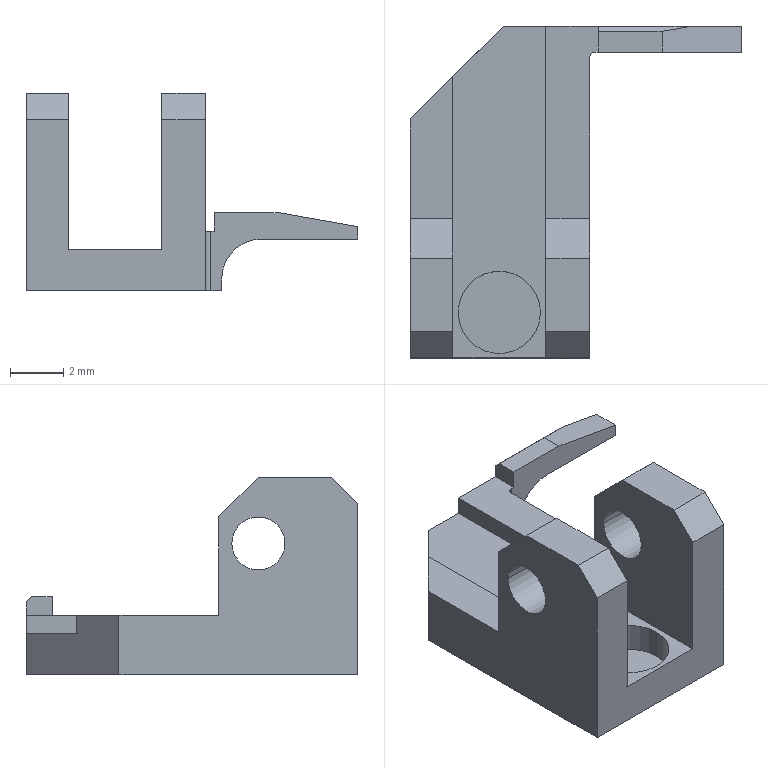Part | NX | 1 solid | 36 faces | box 12.481 x 12.5 x 7.45 mm | volume 217.887 mm3 | plane 28 | cylinder 8 | commonest cylinder face diameters 2 x4 3.1 x2 0.4 x1 3 x1
STEP:
#1=CARTESIAN_POINT('',(-42.479,-42.729,-0.8259));
#2=VERTEX_POINT('',#1);
#3=CARTESIAN_POINT('',(-42.479,-43.716,-0.8259));
#4=VERTEX_POINT('',#3);
#5=CARTESIAN_POINT('',(-42.479,-43.322,-0.8259));
#6=DIRECTION('',(0.,-1.,0.));
#7=VECTOR('',#6,1000.);
#8=LINE('',#5,#7);
#9=EDGE_CURVE('',#2,#4,#8,.T.);
#10=ORIENTED_EDGE('',*,*,#9,.T.);
#11=CARTESIAN_POINT('',(-42.479,-43.716,-1.297));
#12=VERTEX_POINT('',#11);
#13=CARTESIAN_POINT('',(-42.479,-43.716,-2.097));
#14=DIRECTION('',(0.,0.,1.));
#15=VECTOR('',#14,1000.);
#16=LINE('',#13,#15);
#17=EDGE_CURVE('',#12,#4,#16,.T.);
#18=ORIENTED_EDGE('',*,*,#17,.F.);
#19=CARTESIAN_POINT('',(-42.479,-42.729,-1.297));
#20=VERTEX_POINT('',#19);
#21=CARTESIAN_POINT('',(-42.479,-42.161,-1.297));
#22=DIRECTION('',(0.,1.,0.));
#23=VECTOR('',#22,1000.);
#24=LINE('',#21,#23);
#25=EDGE_CURVE('',#12,#20,#24,.T.);
#26=ORIENTED_EDGE('',*,*,#25,.T.);
#27=CARTESIAN_POINT('',(-42.479,-42.729,-2.097));
#28=DIRECTION('',(0.,0.,-1.));
#29=VECTOR('',#28,1000.);
#30=LINE('',#27,#29);
#31=EDGE_CURVE('',#2,#20,#30,.T.);
#32=ORIENTED_EDGE('',*,*,#31,.F.);
#33=EDGE_LOOP('',(#10,#18,#26,#32));
#34=FACE_BOUND('',#33,.T.);
#35=CARTESIAN_POINT('',(-42.479,-43.677,-2.097));
#36=DIRECTION('',(1.,0.,0.));
#37=DIRECTION('',(0.,0.,1.));
#38=AXIS2_PLACEMENT_3D('',#35,#36,#37);
#39=PLANE('',#38);
#40=ADVANCED_FACE('',(#34),#39,.T.);
#41=CARTESIAN_POINT('',(-47.879,-43.716,-0.9969));
#42=VERTEX_POINT('',#41);
#43=CARTESIAN_POINT('',(-47.879,-43.716,-0.2969));
#44=VERTEX_POINT('',#43);
#45=CARTESIAN_POINT('',(-47.879,-43.716,-2.097));
#46=DIRECTION('',(0.,0.,1.));
#47=VECTOR('',#46,1000.);
#48=LINE('',#45,#47);
#49=EDGE_CURVE('',#42,#44,#48,.T.);
#50=ORIENTED_EDGE('',*,*,#49,.T.);
#51=CARTESIAN_POINT('',(-47.879,-42.929,-0.2969));
#52=VERTEX_POINT('',#51);
#53=CARTESIAN_POINT('',(-47.879,-42.161,-0.2969));
#54=DIRECTION('',(0.,-1.,0.));
#55=VECTOR('',#54,1000.);
#56=LINE('',#53,#55);
#57=EDGE_CURVE('',#52,#44,#56,.T.);
#58=ORIENTED_EDGE('',*,*,#57,.F.);
#59=CARTESIAN_POINT('',(-47.879,-42.729,-0.4969));
#60=VERTEX_POINT('',#59);
#61=CARTESIAN_POINT('',(-47.879,-42.161,-1.065));
#62=DIRECTION('',(0.,0.7071,-0.7071));
#63=VECTOR('',#62,1000.);
#64=LINE('',#61,#63);
#65=EDGE_CURVE('',#52,#60,#64,.T.);
#66=ORIENTED_EDGE('',*,*,#65,.T.);
#67=CARTESIAN_POINT('',(-47.879,-42.729,-0.9969));
#68=VERTEX_POINT('',#67);
#69=CARTESIAN_POINT('',(-47.879,-42.729,-2.097));
#70=DIRECTION('',(0.,0.,-1.));
#71=VECTOR('',#70,1000.);
#72=LINE('',#69,#71);
#73=EDGE_CURVE('',#60,#68,#72,.T.);
#74=ORIENTED_EDGE('',*,*,#73,.T.);
#75=CARTESIAN_POINT('',(-47.879,-42.161,-0.9969));
#76=DIRECTION('',(0.,-1.,0.));
#77=VECTOR('',#76,1000.);
#78=LINE('',#75,#77);
#79=EDGE_CURVE('',#68,#42,#78,.T.);
#80=ORIENTED_EDGE('',*,*,#79,.T.);
#81=EDGE_LOOP('',(#50,#58,#66,#74,#80));
#82=FACE_BOUND('',#81,.T.);
#83=CARTESIAN_POINT('',(-47.879,-42.677,-2.097));
#84=DIRECTION('',(-1.,0.,0.));
#85=DIRECTION('',(0.,1.,0.));
#86=AXIS2_PLACEMENT_3D('',#83,#84,#85);
#87=PLANE('',#86);
#88=ADVANCED_FACE('',(#82),#87,.T.);
#89=CARTESIAN_POINT('',(-53.36,-55.229,-1.697));
#90=VERTEX_POINT('',#89);
#91=CARTESIAN_POINT('',(-53.36,-55.229,3.203));
#92=VERTEX_POINT('',#91);
#93=CARTESIAN_POINT('',(-53.36,-55.229,-2.097));
#94=DIRECTION('',(0.,0.,1.));
#95=VECTOR('',#94,1000.);
#96=LINE('',#93,#95);
#97=EDGE_CURVE('',#90,#92,#96,.T.);
#98=ORIENTED_EDGE('',*,*,#97,.F.);
#99=CARTESIAN_POINT('',(-53.36,-44.629,-1.697));
#100=VERTEX_POINT('',#99);
#101=CARTESIAN_POINT('',(-53.36,-42.161,-1.697));
#102=DIRECTION('',(0.,-1.,0.));
#103=VECTOR('',#102,1000.);
#104=LINE('',#101,#103);
#105=EDGE_CURVE('',#100,#90,#104,.T.);
#106=ORIENTED_EDGE('',*,*,#105,.F.);
#107=CARTESIAN_POINT('',(-53.36,-44.629,-0.9969));
#108=VERTEX_POINT('',#107);
#109=CARTESIAN_POINT('',(-53.36,-44.629,-2.097));
#110=DIRECTION('',(0.,0.,-1.));
#111=VECTOR('',#110,1000.);
#112=LINE('',#109,#111);
#113=EDGE_CURVE('',#108,#100,#112,.T.);
#114=ORIENTED_EDGE('',*,*,#113,.F.);
#115=CARTESIAN_POINT('',(-53.36,-49.979,-0.9969));
#116=VERTEX_POINT('',#115);
#117=CARTESIAN_POINT('',(-53.36,-42.161,-0.9969));
#118=DIRECTION('',(0.,-1.,0.));
#119=VECTOR('',#118,1000.);
#120=LINE('',#117,#119);
#121=EDGE_CURVE('',#108,#116,#120,.T.);
#122=ORIENTED_EDGE('',*,*,#121,.T.);
#123=CARTESIAN_POINT('',(-53.36,-49.979,2.703));
#124=VERTEX_POINT('',#123);
#125=CARTESIAN_POINT('',(-53.36,-49.979,-2.097));
#126=DIRECTION('',(0.,0.,-1.));
#127=VECTOR('',#126,1000.);
#128=LINE('',#125,#127);
#129=EDGE_CURVE('',#124,#116,#128,.T.);
#130=ORIENTED_EDGE('',*,*,#129,.F.);
#131=CARTESIAN_POINT('',(-53.36,-51.479,4.203));
#132=VERTEX_POINT('',#131);
#133=CARTESIAN_POINT('',(-53.36,-45.179,-2.097));
#134=DIRECTION('',(0.,-0.7071,0.7071));
#135=VECTOR('',#134,1000.);
#136=LINE('',#133,#135);
#137=EDGE_CURVE('',#124,#132,#136,.T.);
#138=ORIENTED_EDGE('',*,*,#137,.T.);
#139=CARTESIAN_POINT('',(-53.36,-54.229,4.203));
#140=VERTEX_POINT('',#139);
#141=CARTESIAN_POINT('',(-53.36,-42.161,4.203));
#142=DIRECTION('',(0.,1.,0.));
#143=VECTOR('',#142,1000.);
#144=LINE('',#141,#143);
#145=EDGE_CURVE('',#140,#132,#144,.T.);
#146=ORIENTED_EDGE('',*,*,#145,.F.);
#147=CARTESIAN_POINT('',(-53.36,-60.529,-2.097));
#148=DIRECTION('',(0.,-0.7071,-0.7071));
#149=VECTOR('',#148,1000.);
#150=LINE('',#147,#149);
#151=EDGE_CURVE('',#140,#92,#150,.T.);
#152=ORIENTED_EDGE('',*,*,#151,.T.);
#153=EDGE_LOOP('',(#98,#106,#114,#122,#130,#138,#146,#152));
#154=FACE_BOUND('',#153,.T.);
#155=CARTESIAN_POINT('',(-53.36,-52.479,1.703));
#156=VERTEX_POINT('',#155);
#157=CARTESIAN_POINT('',(-53.36,-50.479,1.703));
#158=VERTEX_POINT('',#157);
#159=CARTESIAN_POINT('',(-53.36,-51.479,1.703));
#160=DIRECTION('',(-1.,0.,0.));
#161=DIRECTION('',(0.,-1.,0.));
#162=AXIS2_PLACEMENT_3D('',#159,#160,#161);
#163=CIRCLE('',#162,1.);
#164=EDGE_CURVE('',#156,#158,#163,.T.);
#165=ORIENTED_EDGE('',*,*,#164,.T.);
#166=CARTESIAN_POINT('',(-53.36,-51.479,1.703));
#167=DIRECTION('',(-1.,0.,0.));
#168=DIRECTION('',(0.,-1.,0.));
#169=AXIS2_PLACEMENT_3D('',#166,#167,#168);
#170=CIRCLE('',#169,1.);
#171=EDGE_CURVE('',#158,#156,#170,.T.);
#172=ORIENTED_EDGE('',*,*,#171,.T.);
#173=EDGE_LOOP('',(#165,#172));
#174=FACE_BOUND('',#173,.T.);
#175=CARTESIAN_POINT('',(-53.36,-41.455,-0.9969));
#176=DIRECTION('',(-1.,0.,0.));
#177=DIRECTION('',(0.,0.,1.));
#178=AXIS2_PLACEMENT_3D('',#175,#176,#177);
#179=PLANE('',#178);
#180=ADVANCED_FACE('',(#154,#174),#179,.F.);
#181=ORIENTED_EDGE('',*,*,#31,.T.);
#182=CARTESIAN_POINT('',(-46.102,-42.729,-1.297));
#183=VERTEX_POINT('',#182);
#184=CARTESIAN_POINT('',(-49.458,-42.729,-1.297));
#185=DIRECTION('',(-1.,0.,0.));
#186=VECTOR('',#185,1000.);
#187=LINE('',#184,#186);
#188=EDGE_CURVE('',#20,#183,#187,.T.);
#189=ORIENTED_EDGE('',*,*,#188,.T.);
#190=CARTESIAN_POINT('',(-47.602,-42.729,-2.797));
#191=VERTEX_POINT('',#190);
#192=CARTESIAN_POINT('',(-46.102,-42.729,-2.797));
#193=DIRECTION('',(0.,1.,0.));
#194=DIRECTION('',(0.,0.,-1.));
#195=AXIS2_PLACEMENT_3D('',#192,#193,#194);
#196=CIRCLE('',#195,1.5);
#197=EDGE_CURVE('',#191,#183,#196,.T.);
#198=ORIENTED_EDGE('',*,*,#197,.F.);
#199=CARTESIAN_POINT('',(-47.602,-42.729,-3.247));
#200=VERTEX_POINT('',#199);
#201=CARTESIAN_POINT('',(-47.602,-42.729,-2.097));
#202=DIRECTION('',(0.,0.,1.));
#203=VECTOR('',#202,1000.);
#204=LINE('',#201,#203);
#205=EDGE_CURVE('',#200,#191,#204,.T.);
#206=ORIENTED_EDGE('',*,*,#205,.F.);
#207=CARTESIAN_POINT('',(-51.46,-42.729,-3.247));
#208=VERTEX_POINT('',#207);
#209=CARTESIAN_POINT('',(-49.458,-42.729,-3.247));
#210=DIRECTION('',(-1.,0.,0.));
#211=VECTOR('',#210,1000.);
#212=LINE('',#209,#211);
#213=EDGE_CURVE('',#200,#208,#212,.T.);
#214=ORIENTED_EDGE('',*,*,#213,.T.);
#215=CARTESIAN_POINT('',(-51.46,-42.729,-1.697));
#216=VERTEX_POINT('',#215);
#217=CARTESIAN_POINT('',(-51.46,-42.729,-2.097));
#218=DIRECTION('',(0.,0.,1.));
#219=VECTOR('',#218,1000.);
#220=LINE('',#217,#219);
#221=EDGE_CURVE('',#208,#216,#220,.T.);
#222=ORIENTED_EDGE('',*,*,#221,.T.);
#223=CARTESIAN_POINT('',(-49.86,-42.729,-1.697));
#224=VERTEX_POINT('',#223);
#225=CARTESIAN_POINT('',(-49.458,-42.729,-1.697));
#226=DIRECTION('',(-1.,0.,0.));
#227=VECTOR('',#226,1000.);
#228=LINE('',#225,#227);
#229=EDGE_CURVE('',#224,#216,#228,.T.);
#230=ORIENTED_EDGE('',*,*,#229,.F.);
#231=CARTESIAN_POINT('',(-49.86,-42.729,-0.9969));
#232=VERTEX_POINT('',#231);
#233=CARTESIAN_POINT('',(-49.86,-42.729,-2.097));
#234=DIRECTION('',(0.,0.,-1.));
#235=VECTOR('',#234,1000.);
#236=LINE('',#233,#235);
#237=EDGE_CURVE('',#232,#224,#236,.T.);
#238=ORIENTED_EDGE('',*,*,#237,.F.);
#239=CARTESIAN_POINT('',(-49.458,-42.729,-0.9969));
#240=DIRECTION('',(-1.,0.,0.));
#241=VECTOR('',#240,1000.);
#242=LINE('',#239,#241);
#243=EDGE_CURVE('',#68,#232,#242,.T.);
#244=ORIENTED_EDGE('',*,*,#243,.F.);
#245=ORIENTED_EDGE('',*,*,#73,.F.);
#246=CARTESIAN_POINT('',(-44.345,-42.729,-0.4969));
#247=VERTEX_POINT('',#246);
#248=CARTESIAN_POINT('',(-49.458,-42.729,-0.4969));
#249=DIRECTION('',(1.,0.,0.));
#250=VECTOR('',#249,1000.);
#251=LINE('',#248,#250);
#252=EDGE_CURVE('',#60,#247,#251,.T.);
#253=ORIENTED_EDGE('',*,*,#252,.T.);
#254=CARTESIAN_POINT('',(-49.458,-42.729,0.4047));
#255=DIRECTION('',(0.9848,0.,-0.1736));
#256=VECTOR('',#255,1000.);
#257=LINE('',#254,#256);
#258=EDGE_CURVE('',#247,#2,#257,.T.);
#259=ORIENTED_EDGE('',*,*,#258,.T.);
#260=EDGE_LOOP('',(#181,#189,#198,#206,#214,#222,#230,#238,#244,#245,#253,#259));
#261=FACE_BOUND('',#260,.T.);
#262=CARTESIAN_POINT('',(-40.479,-42.729,-2.097));
#263=DIRECTION('',(0.,1.,0.));
#264=DIRECTION('',(0.,0.,-1.));
#265=AXIS2_PLACEMENT_3D('',#262,#263,#264);
#266=PLANE('',#265);
#267=ADVANCED_FACE('',(#261),#266,.T.);
#268=CARTESIAN_POINT('',(-48.01,-43.716,-0.9969));
#269=VERTEX_POINT('',#268);
#270=CARTESIAN_POINT('',(-48.01,-43.716,-3.247));
#271=VERTEX_POINT('',#270);
#272=CARTESIAN_POINT('',(-48.01,-43.716,-2.097));
#273=DIRECTION('',(0.,0.,-1.));
#274=VECTOR('',#273,1000.);
#275=LINE('',#272,#274);
#276=EDGE_CURVE('',#269,#271,#275,.T.);
#277=ORIENTED_EDGE('',*,*,#276,.T.);
#278=CARTESIAN_POINT('',(-47.602,-43.716,-3.247));
#279=VERTEX_POINT('',#278);
#280=CARTESIAN_POINT('',(-49.458,-43.716,-3.247));
#281=DIRECTION('',(1.,0.,0.));
#282=VECTOR('',#281,1000.);
#283=LINE('',#280,#282);
#284=EDGE_CURVE('',#271,#279,#283,.T.);
#285=ORIENTED_EDGE('',*,*,#284,.T.);
#286=CARTESIAN_POINT('',(-47.602,-43.716,-2.797));
#287=VERTEX_POINT('',#286);
#288=CARTESIAN_POINT('',(-47.602,-43.716,-2.097));
#289=DIRECTION('',(0.,0.,-1.));
#290=VECTOR('',#289,1000.);
#291=LINE('',#288,#290);
#292=EDGE_CURVE('',#287,#279,#291,.T.);
#293=ORIENTED_EDGE('',*,*,#292,.F.);
#294=CARTESIAN_POINT('',(-46.102,-43.716,-1.297));
#295=VERTEX_POINT('',#294);
#296=CARTESIAN_POINT('',(-46.102,-43.716,-2.797));
#297=DIRECTION('',(0.,-1.,0.));
#298=DIRECTION('',(0.,0.,1.));
#299=AXIS2_PLACEMENT_3D('',#296,#297,#298);
#300=CIRCLE('',#299,1.5);
#301=EDGE_CURVE('',#295,#287,#300,.T.);
#302=ORIENTED_EDGE('',*,*,#301,.F.);
#303=CARTESIAN_POINT('',(-49.458,-43.716,-1.297));
#304=DIRECTION('',(1.,0.,0.));
#305=VECTOR('',#304,1000.);
#306=LINE('',#303,#305);
#307=EDGE_CURVE('',#295,#12,#306,.T.);
#308=ORIENTED_EDGE('',*,*,#307,.T.);
#309=ORIENTED_EDGE('',*,*,#17,.T.);
#310=CARTESIAN_POINT('',(-45.479,-43.716,-0.2969));
#311=VERTEX_POINT('',#310);
#312=CARTESIAN_POINT('',(-49.458,-43.716,0.4047));
#313=DIRECTION('',(-0.9848,0.,0.1736));
#314=VECTOR('',#313,1000.);
#315=LINE('',#312,#314);
#316=EDGE_CURVE('',#4,#311,#315,.T.);
#317=ORIENTED_EDGE('',*,*,#316,.T.);
#318=CARTESIAN_POINT('',(-49.458,-43.716,-0.2969));
#319=DIRECTION('',(-1.,0.,0.));
#320=VECTOR('',#319,1000.);
#321=LINE('',#318,#320);
#322=EDGE_CURVE('',#311,#44,#321,.T.);
#323=ORIENTED_EDGE('',*,*,#322,.T.);
#324=ORIENTED_EDGE('',*,*,#49,.F.);
#325=CARTESIAN_POINT('',(-49.458,-43.716,-0.9969));
#326=DIRECTION('',(1.,0.,0.));
#327=VECTOR('',#326,1000.);
#328=LINE('',#325,#327);
#329=EDGE_CURVE('',#269,#42,#328,.T.);
#330=ORIENTED_EDGE('',*,*,#329,.F.);
#331=EDGE_LOOP('',(#277,#285,#293,#302,#308,#309,#317,#323,#324,#330));
#332=FACE_BOUND('',#331,.T.);
#333=CARTESIAN_POINT('',(-49.857,-43.716,-2.975));
#334=DIRECTION('',(0.,-1.,0.));
#335=DIRECTION('',(-1.,0.,0.));
#336=AXIS2_PLACEMENT_3D('',#333,#334,#335);
#337=PLANE('',#336);
#338=ADVANCED_FACE('',(#332),#337,.T.);
#339=CARTESIAN_POINT('',(-48.21,-55.229,-3.247));
#340=VERTEX_POINT('',#339);
#341=CARTESIAN_POINT('',(-48.21,-55.229,3.203));
#342=VERTEX_POINT('',#341);
#343=CARTESIAN_POINT('',(-48.21,-55.229,-2.097));
#344=DIRECTION('',(0.,0.,1.));
#345=VECTOR('',#344,1000.);
#346=LINE('',#343,#345);
#347=EDGE_CURVE('',#340,#342,#346,.T.);
#348=ORIENTED_EDGE('',*,*,#347,.T.);
#349=CARTESIAN_POINT('',(-49.86,-55.229,3.203));
#350=VERTEX_POINT('',#349);
#351=CARTESIAN_POINT('',(-49.035,-55.229,3.203));
#352=DIRECTION('',(1.,0.,0.));
#353=VECTOR('',#352,1000.);
#354=LINE('',#351,#353);
#355=EDGE_CURVE('',#350,#342,#354,.T.);
#356=ORIENTED_EDGE('',*,*,#355,.F.);
#357=CARTESIAN_POINT('',(-49.86,-55.229,-1.697));
#358=VERTEX_POINT('',#357);
#359=CARTESIAN_POINT('',(-49.86,-55.229,-2.097));
#360=DIRECTION('',(0.,0.,-1.));
#361=VECTOR('',#360,1000.);
#362=LINE('',#359,#361);
#363=EDGE_CURVE('',#350,#358,#362,.T.);
#364=ORIENTED_EDGE('',*,*,#363,.T.);
#365=CARTESIAN_POINT('',(-49.458,-55.229,-1.697));
#366=DIRECTION('',(-1.,0.,0.));
#367=VECTOR('',#366,1000.);
#368=LINE('',#365,#367);
#369=EDGE_CURVE('',#358,#90,#368,.T.);
#370=ORIENTED_EDGE('',*,*,#369,.T.);
#371=ORIENTED_EDGE('',*,*,#97,.T.);
#372=CARTESIAN_POINT('',(-54.96,-55.229,3.203));
#373=VERTEX_POINT('',#372);
#374=CARTESIAN_POINT('',(-54.16,-55.229,3.203));
#375=DIRECTION('',(1.,0.,0.));
#376=VECTOR('',#375,1000.);
#377=LINE('',#374,#376);
#378=EDGE_CURVE('',#373,#92,#377,.T.);
#379=ORIENTED_EDGE('',*,*,#378,.F.);
#380=CARTESIAN_POINT('',(-54.96,-55.229,-3.247));
#381=VERTEX_POINT('',#380);
#382=CARTESIAN_POINT('',(-54.96,-55.229,-2.097));
#383=DIRECTION('',(0.,0.,1.));
#384=VECTOR('',#383,1000.);
#385=LINE('',#382,#384);
#386=EDGE_CURVE('',#381,#373,#385,.T.);
#387=ORIENTED_EDGE('',*,*,#386,.F.);
#388=CARTESIAN_POINT('',(-49.458,-55.229,-3.247));
#389=DIRECTION('',(-1.,0.,0.));
#390=VECTOR('',#389,1000.);
#391=LINE('',#388,#390);
#392=EDGE_CURVE('',#340,#381,#391,.T.);
#393=ORIENTED_EDGE('',*,*,#392,.F.);
#394=EDGE_LOOP('',(#348,#356,#364,#370,#371,#379,#387,#393));
#395=FACE_BOUND('',#394,.T.);
#396=CARTESIAN_POINT('',(-46.479,-55.229,-2.097));
#397=DIRECTION('',(0.,-1.,0.));
#398=DIRECTION('',(-1.,0.,0.));
#399=AXIS2_PLACEMENT_3D('',#396,#397,#398);
#400=PLANE('',#399);
#401=ADVANCED_FACE('',(#395),#400,.T.);
#402=CARTESIAN_POINT('',(-47.602,-45.216,-2.797));
#403=DIRECTION('',(0.,1.,0.));
#404=VECTOR('',#403,1000.);
#405=LINE('',#402,#404);
#406=EDGE_CURVE('',#287,#191,#405,.T.);
#407=ORIENTED_EDGE('',*,*,#406,.F.);
#408=ORIENTED_EDGE('',*,*,#292,.T.);
#409=CARTESIAN_POINT('',(-47.602,-42.161,-3.247));
#410=DIRECTION('',(0.,-1.,0.));
#411=VECTOR('',#410,1000.);
#412=LINE('',#409,#411);
#413=EDGE_CURVE('',#200,#279,#412,.T.);
#414=ORIENTED_EDGE('',*,*,#413,.F.);
#415=ORIENTED_EDGE('',*,*,#205,.T.);
#416=EDGE_LOOP('',(#407,#408,#414,#415));
#417=FACE_BOUND('',#416,.T.);
#418=CARTESIAN_POINT('',(-47.602,-42.161,-2.747));
#419=DIRECTION('',(-1.,0.,0.));
#420=DIRECTION('',(0.,0.,1.));
#421=AXIS2_PLACEMENT_3D('',#418,#419,#420);
#422=PLANE('',#421);
#423=ADVANCED_FACE('',(#417),#422,.F.);
#424=ORIENTED_EDGE('',*,*,#406,.T.);
#425=ORIENTED_EDGE('',*,*,#197,.T.);
#426=CARTESIAN_POINT('',(-46.102,-45.216,-1.297));
#427=DIRECTION('',(0.,1.,0.));
#428=VECTOR('',#427,1000.);
#429=LINE('',#426,#428);
#430=EDGE_CURVE('',#295,#183,#429,.T.);
#431=ORIENTED_EDGE('',*,*,#430,.F.);
#432=ORIENTED_EDGE('',*,*,#301,.T.);
#433=EDGE_LOOP('',(#424,#425,#431,#432));
#434=FACE_BOUND('',#433,.T.);
#435=CARTESIAN_POINT('',(-46.102,-45.216,-2.797));
#436=DIRECTION('',(0.,1.,0.));
#437=DIRECTION('',(1.,0.,0.));
#438=AXIS2_PLACEMENT_3D('',#435,#436,#437);
#439=CYLINDRICAL_SURFACE('',#438,1.5);
#440=ADVANCED_FACE('',(#434),#439,.F.);
#441=ORIENTED_EDGE('',*,*,#276,.F.);
#442=CARTESIAN_POINT('',(-48.21,-43.916,-0.9969));
#443=VERTEX_POINT('',#442);
#444=CARTESIAN_POINT('',(-48.01,-43.916,-0.9969));
#445=DIRECTION('',(0.,0.,-1.));
#446=DIRECTION('',(-1.,0.,0.));
#447=AXIS2_PLACEMENT_3D('',#444,#445,#446);
#448=CIRCLE('',#447,0.2);
#449=EDGE_CURVE('',#443,#269,#448,.T.);
#450=ORIENTED_EDGE('',*,*,#449,.F.);
#451=CARTESIAN_POINT('',(-48.21,-43.916,-3.247));
#452=VERTEX_POINT('',#451);
#453=CARTESIAN_POINT('',(-48.21,-43.916,-2.097));
#454=DIRECTION('',(0.,0.,-1.));
#455=VECTOR('',#454,1000.);
#456=LINE('',#453,#455);
#457=EDGE_CURVE('',#443,#452,#456,.T.);
#458=ORIENTED_EDGE('',*,*,#457,.T.);
#459=CARTESIAN_POINT('',(-48.01,-43.916,-3.247));
#460=DIRECTION('',(0.,0.,-1.));
#461=DIRECTION('',(-1.,0.,0.));
#462=AXIS2_PLACEMENT_3D('',#459,#460,#461);
#463=CIRCLE('',#462,0.2);
#464=EDGE_CURVE('',#452,#271,#463,.T.);
#465=ORIENTED_EDGE('',*,*,#464,.T.);
#466=EDGE_LOOP('',(#441,#450,#458,#465));
#467=FACE_BOUND('',#466,.T.);
#468=CARTESIAN_POINT('',(-48.01,-43.916,-2.097));
#469=DIRECTION('',(0.,0.,-1.));
#470=DIRECTION('',(-1.,0.,0.));
#471=AXIS2_PLACEMENT_3D('',#468,#469,#470);
#472=CYLINDRICAL_SURFACE('',#471,0.2);
#473=ADVANCED_FACE('',(#467),#472,.F.);
#474=ORIENTED_EDGE('',*,*,#164,.F.);
#475=CARTESIAN_POINT('',(-54.96,-52.479,1.703));
#476=VERTEX_POINT('',#475);
#477=CARTESIAN_POINT('',(-40.131,-52.479,1.703));
#478=DIRECTION('',(-1.,0.,0.));
#479=VECTOR('',#478,1000.);
#480=LINE('',#477,#479);
#481=EDGE_CURVE('',#476,#156,#480,.F.);
#482=ORIENTED_EDGE('',*,*,#481,.F.);
#483=CARTESIAN_POINT('',(-54.96,-50.479,1.703));
#484=VERTEX_POINT('',#483);
#485=CARTESIAN_POINT('',(-54.96,-51.479,1.703));
#486=DIRECTION('',(-1.,0.,0.));
#487=DIRECTION('',(0.,-1.,0.));
#488=AXIS2_PLACEMENT_3D('',#485,#486,#487);
#489=CIRCLE('',#488,1.);
#490=EDGE_CURVE('',#476,#484,#489,.T.);
#491=ORIENTED_EDGE('',*,*,#490,.T.);
#492=CARTESIAN_POINT('',(-40.131,-50.479,1.703));
#493=DIRECTION('',(-1.,0.,0.));
#494=VECTOR('',#493,1000.);
#495=LINE('',#492,#494);
#496=EDGE_CURVE('',#484,#158,#495,.F.);
#497=ORIENTED_EDGE('',*,*,#496,.T.);
#498=EDGE_LOOP('',(#474,#482,#491,#497));
#499=FACE_BOUND('',#498,.T.);
#500=CARTESIAN_POINT('',(-40.131,-51.479,1.703));
#501=DIRECTION('',(-1.,0.,0.));
#502=DIRECTION('',(0.,-1.,0.));
#503=AXIS2_PLACEMENT_3D('',#500,#501,#502);
#504=CYLINDRICAL_SURFACE('',#503,1.);
#505=ADVANCED_FACE('',(#499),#504,.F.);
#506=CARTESIAN_POINT('',(-45.479,-42.929,-0.2969));
#507=VERTEX_POINT('',#506);
#508=CARTESIAN_POINT('',(-45.479,-43.322,-0.2969));
#509=DIRECTION('',(0.,-1.,0.));
#510=VECTOR('',#509,1000.);
#511=LINE('',#508,#510);
#512=EDGE_CURVE('',#507,#311,#511,.T.);
#513=ORIENTED_EDGE('',*,*,#512,.T.);
#514=ORIENTED_EDGE('',*,*,#316,.F.);
#515=ORIENTED_EDGE('',*,*,#9,.F.);
#516=ORIENTED_EDGE('',*,*,#258,.F.);
#517=CARTESIAN_POINT('',(-49.458,-43.631,0.4047));
#518=DIRECTION('',(-0.9703,-0.1711,0.1711));
#519=VECTOR('',#518,1000.);
#520=LINE('',#517,#519);
#521=EDGE_CURVE('',#247,#507,#520,.T.);
#522=ORIENTED_EDGE('',*,*,#521,.T.);
#523=EDGE_LOOP('',(#513,#514,#515,#516,#522));
#524=FACE_BOUND('',#523,.T.);
#525=CARTESIAN_POINT('',(-43.979,-43.322,-0.5614));
#526=DIRECTION('',(-0.1736,0.,-0.9848));
#527=DIRECTION('',(-0.9848,0.,0.1736));
#528=AXIS2_PLACEMENT_3D('',#525,#526,#527);
#529=PLANE('',#528);
#530=ADVANCED_FACE('',(#524),#529,.F.);
#531=ORIENTED_EDGE('',*,*,#284,.F.);
#532=ORIENTED_EDGE('',*,*,#464,.F.);
#533=CARTESIAN_POINT('',(-48.21,-42.161,-3.247));
#534=DIRECTION('',(0.,1.,0.));
#535=VECTOR('',#534,1000.);
#536=LINE('',#533,#535);
#537=EDGE_CURVE('',#340,#452,#536,.T.);
#538=ORIENTED_EDGE('',*,*,#537,.F.);
#539=ORIENTED_EDGE('',*,*,#392,.T.);
#540=CARTESIAN_POINT('',(-54.96,-46.229,-3.247));
#541=VERTEX_POINT('',#540);
#542=CARTESIAN_POINT('',(-54.96,-42.161,-3.247));
#543=DIRECTION('',(0.,-1.,0.));
#544=VECTOR('',#543,1000.);
#545=LINE('',#542,#544);
#546=EDGE_CURVE('',#541,#381,#545,.T.);
#547=ORIENTED_EDGE('',*,*,#546,.F.);
#548=CARTESIAN_POINT('',(-50.893,-42.161,-3.247));
#549=DIRECTION('',(0.7071,0.7071,0.));
#550=VECTOR('',#549,1000.);
#551=LINE('',#548,#550);
#552=EDGE_CURVE('',#541,#208,#551,.T.);
#553=ORIENTED_EDGE('',*,*,#552,.T.);
#554=ORIENTED_EDGE('',*,*,#213,.F.);
#555=ORIENTED_EDGE('',*,*,#413,.T.);
#556=EDGE_LOOP('',(#531,#532,#538,#539,#547,#553,#554,#555));
#557=FACE_BOUND('',#556,.T.);
#558=CARTESIAN_POINT('',(-49.458,-42.161,-3.247));
#559=DIRECTION('',(0.,0.,-1.));
#560=DIRECTION('',(0.,-1.,0.));
#561=AXIS2_PLACEMENT_3D('',#558,#559,#560);
#562=PLANE('',#561);
#563=ADVANCED_FACE('',(#557),#562,.T.);
#564=CARTESIAN_POINT('',(-54.96,-46.229,-0.9969));
#565=VERTEX_POINT('',#564);
#566=CARTESIAN_POINT('',(-54.96,-46.229,-2.097));
#567=DIRECTION('',(0.,0.,1.));
#568=VECTOR('',#567,1000.);
#569=LINE('',#566,#568);
#570=EDGE_CURVE('',#541,#565,#569,.T.);
#571=ORIENTED_EDGE('',*,*,#570,.F.);
#572=ORIENTED_EDGE('',*,*,#546,.T.);
#573=ORIENTED_EDGE('',*,*,#386,.T.);
#574=CARTESIAN_POINT('',(-54.96,-54.229,4.203));
#575=VERTEX_POINT('',#574);
#576=CARTESIAN_POINT('',(-54.96,-60.529,-2.097));
#577=DIRECTION('',(0.,-0.7071,-0.7071));
#578=VECTOR('',#577,1000.);
#579=LINE('',#576,#578);
#580=EDGE_CURVE('',#575,#373,#579,.T.);
#581=ORIENTED_EDGE('',*,*,#580,.F.);
#582=CARTESIAN_POINT('',(-54.96,-51.479,4.203));
#583=VERTEX_POINT('',#582);
#584=CARTESIAN_POINT('',(-54.96,-42.161,4.203));
#585=DIRECTION('',(0.,1.,0.));
#586=VECTOR('',#585,1000.);
#587=LINE('',#584,#586);
#588=EDGE_CURVE('',#575,#583,#587,.T.);
#589=ORIENTED_EDGE('',*,*,#588,.T.);
#590=CARTESIAN_POINT('',(-54.96,-49.979,2.703));
#591=VERTEX_POINT('',#590);
#592=CARTESIAN_POINT('',(-54.96,-45.179,-2.097));
#593=DIRECTION('',(0.,-0.7071,0.7071));
#594=VECTOR('',#593,1000.);
#595=LINE('',#592,#594);
#596=EDGE_CURVE('',#591,#583,#595,.T.);
#597=ORIENTED_EDGE('',*,*,#596,.F.);
#598=CARTESIAN_POINT('',(-54.96,-49.979,-0.9969));
#599=VERTEX_POINT('',#598);
#600=CARTESIAN_POINT('',(-54.96,-49.979,-2.097));
#601=DIRECTION('',(0.,0.,-1.));
#602=VECTOR('',#601,1000.);
#603=LINE('',#600,#602);
#604=EDGE_CURVE('',#591,#599,#603,.T.);
#605=ORIENTED_EDGE('',*,*,#604,.T.);
#606=CARTESIAN_POINT('',(-54.96,-42.161,-0.9969));
#607=DIRECTION('',(0.,-1.,0.));
#608=VECTOR('',#607,1000.);
#609=LINE('',#606,#608);
#610=EDGE_CURVE('',#565,#599,#609,.T.);
#611=ORIENTED_EDGE('',*,*,#610,.F.);
#612=EDGE_LOOP('',(#571,#572,#573,#581,#589,#597,#605,#611));
#613=FACE_BOUND('',#612,.T.);
#614=CARTESIAN_POINT('',(-54.96,-51.479,1.703));
#615=DIRECTION('',(-1.,0.,0.));
#616=DIRECTION('',(0.,-1.,0.));
#617=AXIS2_PLACEMENT_3D('',#614,#615,#616);
#618=CIRCLE('',#617,1.);
#619=EDGE_CURVE('',#484,#476,#618,.T.);
#620=ORIENTED_EDGE('',*,*,#619,.F.);
#621=ORIENTED_EDGE('',*,*,#490,.F.);
#622=EDGE_LOOP('',(#620,#621));
#623=FACE_BOUND('',#622,.T.);
#624=CARTESIAN_POINT('',(-54.96,-43.105,-3.373));
#625=DIRECTION('',(-1.,0.,0.));
#626=DIRECTION('',(0.,1.,0.));
#627=AXIS2_PLACEMENT_3D('',#624,#625,#626);
#628=PLANE('',#627);
#629=ADVANCED_FACE('',(#613,#623),#628,.T.);
#630=ORIENTED_EDGE('',*,*,#79,.F.);
#631=ORIENTED_EDGE('',*,*,#243,.T.);
#632=CARTESIAN_POINT('',(-49.86,-49.979,-0.9969));
#633=VERTEX_POINT('',#632);
#634=CARTESIAN_POINT('',(-49.86,-42.161,-0.9969));
#635=DIRECTION('',(0.,1.,0.));
#636=VECTOR('',#635,1000.);
#637=LINE('',#634,#636);
#638=EDGE_CURVE('',#633,#232,#637,.T.);
#639=ORIENTED_EDGE('',*,*,#638,.F.);
#640=CARTESIAN_POINT('',(-48.21,-49.979,-0.9969));
#641=VERTEX_POINT('',#640);
#642=CARTESIAN_POINT('',(-49.458,-49.979,-0.9969));
#643=DIRECTION('',(-1.,0.,0.));
#644=VECTOR('',#643,1000.);
#645=LINE('',#642,#644);
#646=EDGE_CURVE('',#641,#633,#645,.T.);
#647=ORIENTED_EDGE('',*,*,#646,.F.);
#648=CARTESIAN_POINT('',(-48.21,-42.161,-0.9969));
#649=DIRECTION('',(0.,-1.,0.));
#650=VECTOR('',#649,1000.);
#651=LINE('',#648,#650);
#652=EDGE_CURVE('',#443,#641,#651,.T.);
#653=ORIENTED_EDGE('',*,*,#652,.F.);
#654=ORIENTED_EDGE('',*,*,#449,.T.);
#655=ORIENTED_EDGE('',*,*,#329,.T.);
#656=EDGE_LOOP('',(#630,#631,#639,#647,#653,#654,#655));
#657=FACE_BOUND('',#656,.T.);
#658=CARTESIAN_POINT('',(-46.479,-42.677,-0.9969));
#659=DIRECTION('',(0.,0.,1.));
#660=DIRECTION('',(1.,0.,0.));
#661=AXIS2_PLACEMENT_3D('',#658,#659,#660);
#662=PLANE('',#661);
#663=ADVANCED_FACE('',(#657),#662,.T.);
#664=ORIENTED_EDGE('',*,*,#537,.T.);
#665=ORIENTED_EDGE('',*,*,#457,.F.);
#666=ORIENTED_EDGE('',*,*,#652,.T.);
#667=CARTESIAN_POINT('',(-48.21,-49.979,2.703));
#668=VERTEX_POINT('',#667);
#669=CARTESIAN_POINT('',(-48.21,-49.979,-2.097));
#670=DIRECTION('',(0.,0.,-1.));
#671=VECTOR('',#670,1000.);
#672=LINE('',#669,#671);
#673=EDGE_CURVE('',#668,#641,#672,.T.);
#674=ORIENTED_EDGE('',*,*,#673,.F.);
#675=CARTESIAN_POINT('',(-48.21,-51.479,4.203));
#676=VERTEX_POINT('',#675);
#677=CARTESIAN_POINT('',(-48.21,-45.179,-2.097));
#678=DIRECTION('',(0.,-0.7071,0.7071));
#679=VECTOR('',#678,1000.);
#680=LINE('',#677,#679);
#681=EDGE_CURVE('',#668,#676,#680,.T.);
#682=ORIENTED_EDGE('',*,*,#681,.T.);
#683=CARTESIAN_POINT('',(-48.21,-54.229,4.203));
#684=VERTEX_POINT('',#683);
#685=CARTESIAN_POINT('',(-48.21,-42.161,4.203));
#686=DIRECTION('',(0.,-1.,0.));
#687=VECTOR('',#686,1000.);
#688=LINE('',#685,#687);
#689=EDGE_CURVE('',#676,#684,#688,.T.);
#690=ORIENTED_EDGE('',*,*,#689,.T.);
#691=CARTESIAN_POINT('',(-48.21,-60.529,-2.097));
#692=DIRECTION('',(0.,-0.7071,-0.7071));
#693=VECTOR('',#692,1000.);
#694=LINE('',#691,#693);
#695=EDGE_CURVE('',#684,#342,#694,.T.);
#696=ORIENTED_EDGE('',*,*,#695,.T.);
#697=ORIENTED_EDGE('',*,*,#347,.F.);
#698=EDGE_LOOP('',(#664,#665,#666,#674,#682,#690,#696,#697));
#699=FACE_BOUND('',#698,.T.);
#700=CARTESIAN_POINT('',(-48.21,-50.479,1.703));
#701=VERTEX_POINT('',#700);
#702=CARTESIAN_POINT('',(-48.21,-52.479,1.703));
#703=VERTEX_POINT('',#702);
#704=CARTESIAN_POINT('',(-48.21,-51.479,1.703));
#705=DIRECTION('',(-1.,0.,0.));
#706=DIRECTION('',(0.,-1.,0.));
#707=AXIS2_PLACEMENT_3D('',#704,#705,#706);
#708=CIRCLE('',#707,1.);
#709=EDGE_CURVE('',#701,#703,#708,.T.);
#710=ORIENTED_EDGE('',*,*,#709,.T.);
#711=CARTESIAN_POINT('',(-48.21,-51.479,1.703));
#712=DIRECTION('',(-1.,0.,0.));
#713=DIRECTION('',(0.,-1.,0.));
#714=AXIS2_PLACEMENT_3D('',#711,#712,#713);
#715=CIRCLE('',#714,1.);
#716=EDGE_CURVE('',#703,#701,#715,.T.);
#717=ORIENTED_EDGE('',*,*,#716,.T.);
#718=EDGE_LOOP('',(#710,#717));
#719=FACE_BOUND('',#718,.T.);
#720=CARTESIAN_POINT('',(-48.21,-45.316,3.503));
#721=DIRECTION('',(-1.,0.,0.));
#722=DIRECTION('',(0.,0.,1.));
#723=AXIS2_PLACEMENT_3D('',#720,#721,#722);
#724=PLANE('',#723);
#725=ADVANCED_FACE('',(#699,#719),#724,.F.);
#726=ORIENTED_EDGE('',*,*,#570,.T.);
#727=CARTESIAN_POINT('',(-50.893,-42.161,-0.9969));
#728=DIRECTION('',(0.7071,0.7071,0.));
#729=VECTOR('',#728,1000.);
#730=LINE('',#727,#729);
#731=EDGE_CURVE('',#565,#108,#730,.T.);
#732=ORIENTED_EDGE('',*,*,#731,.T.);
#733=ORIENTED_EDGE('',*,*,#113,.T.);
#734=CARTESIAN_POINT('',(-50.893,-42.161,-1.697));
#735=DIRECTION('',(0.7071,0.7071,0.));
#736=VECTOR('',#735,1000.);
#737=LINE('',#734,#736);
#738=EDGE_CURVE('',#100,#216,#737,.T.);
#739=ORIENTED_EDGE('',*,*,#738,.T.);
#740=ORIENTED_EDGE('',*,*,#221,.F.);
#741=ORIENTED_EDGE('',*,*,#552,.F.);
#742=EDGE_LOOP('',(#726,#732,#733,#739,#740,#741));
#743=FACE_BOUND('',#742,.T.);
#744=CARTESIAN_POINT('',(-53.21,-44.479,-1.872));
#745=DIRECTION('',(0.7071,-0.7071,0.));
#746=DIRECTION('',(0.,0.,-1.));
#747=AXIS2_PLACEMENT_3D('',#744,#745,#746);
#748=PLANE('',#747);
#749=ADVANCED_FACE('',(#743),#748,.F.);
#750=ORIENTED_EDGE('',*,*,#121,.F.);
#751=ORIENTED_EDGE('',*,*,#731,.F.);
#752=ORIENTED_EDGE('',*,*,#610,.T.);
#753=CARTESIAN_POINT('',(-49.458,-49.979,-0.9969));
#754=DIRECTION('',(-1.,0.,0.));
#755=VECTOR('',#754,1000.);
#756=LINE('',#753,#755);
#757=EDGE_CURVE('',#116,#599,#756,.T.);
#758=ORIENTED_EDGE('',*,*,#757,.F.);
#759=EDGE_LOOP('',(#750,#751,#752,#758));
#760=FACE_BOUND('',#759,.T.);
#761=CARTESIAN_POINT('',(-46.479,-42.677,-0.9969));
#762=DIRECTION('',(0.,0.,1.));
#763=DIRECTION('',(1.,0.,0.));
#764=AXIS2_PLACEMENT_3D('',#761,#762,#763);
#765=PLANE('',#764);
#766=ADVANCED_FACE('',(#760),#765,.T.);
#767=CARTESIAN_POINT('',(-53.16,-53.51,-2.797));
#768=VERTEX_POINT('',#767);
#769=CARTESIAN_POINT('',(-50.06,-53.51,-2.797));
#770=VERTEX_POINT('',#769);
#771=CARTESIAN_POINT('',(-51.61,-53.51,-2.797));
#772=DIRECTION('',(0.,0.,-1.));
#773=DIRECTION('',(-1.,0.,0.));
#774=AXIS2_PLACEMENT_3D('',#771,#772,#773);
#775=CIRCLE('',#774,1.55);
#776=EDGE_CURVE('',#768,#770,#775,.T.);
#777=ORIENTED_EDGE('',*,*,#776,.F.);
#778=CARTESIAN_POINT('',(-51.61,-53.51,-2.797));
#779=DIRECTION('',(0.,0.,-1.));
#780=DIRECTION('',(-1.,0.,0.));
#781=AXIS2_PLACEMENT_3D('',#778,#779,#780);
#782=CIRCLE('',#781,1.55);
#783=EDGE_CURVE('',#770,#768,#782,.T.);
#784=ORIENTED_EDGE('',*,*,#783,.F.);
#785=EDGE_LOOP('',(#777,#784));
#786=FACE_BOUND('',#785,.T.);
#787=CARTESIAN_POINT('',(-51.303,-54.872,-2.797));
#788=DIRECTION('',(0.,0.,1.));
#789=DIRECTION('',(1.,0.,0.));
#790=AXIS2_PLACEMENT_3D('',#787,#788,#789);
#791=PLANE('',#790);
#792=ADVANCED_FACE('',(#786),#791,.T.);
#793=ORIENTED_EDGE('',*,*,#512,.F.);
#794=CARTESIAN_POINT('',(-49.458,-42.929,-0.2969));
#795=DIRECTION('',(1.,0.,0.));
#796=VECTOR('',#795,1000.);
#797=LINE('',#794,#796);
#798=EDGE_CURVE('',#52,#507,#797,.T.);
#799=ORIENTED_EDGE('',*,*,#798,.F.);
#800=ORIENTED_EDGE('',*,*,#57,.T.);
#801=ORIENTED_EDGE('',*,*,#322,.F.);
#802=EDGE_LOOP('',(#793,#799,#800,#801));
#803=FACE_BOUND('',#802,.T.);
#804=CARTESIAN_POINT('',(-49.458,-42.161,-0.2969));
#805=DIRECTION('',(0.,0.,-1.));
#806=DIRECTION('',(0.,-1.,0.));
#807=AXIS2_PLACEMENT_3D('',#804,#805,#806);
#808=PLANE('',#807);
#809=ADVANCED_FACE('',(#803),#808,.F.);
#810=ORIENTED_EDGE('',*,*,#430,.T.);
#811=ORIENTED_EDGE('',*,*,#188,.F.);
#812=ORIENTED_EDGE('',*,*,#25,.F.);
#813=ORIENTED_EDGE('',*,*,#307,.F.);
#814=EDGE_LOOP('',(#810,#811,#812,#813));
#815=FACE_BOUND('',#814,.T.);
#816=CARTESIAN_POINT('',(-35.479,-43.777,-1.297));
#817=DIRECTION('',(0.,0.,1.));
#818=DIRECTION('',(0.,-1.,0.));
#819=AXIS2_PLACEMENT_3D('',#816,#817,#818);
#820=PLANE('',#819);
#821=ADVANCED_FACE('',(#815),#820,.F.);
#822=ORIENTED_EDGE('',*,*,#798,.T.);
#823=ORIENTED_EDGE('',*,*,#521,.F.);
#824=ORIENTED_EDGE('',*,*,#252,.F.);
#825=ORIENTED_EDGE('',*,*,#65,.F.);
#826=EDGE_LOOP('',(#822,#823,#824,#825));
#827=FACE_BOUND('',#826,.T.);
#828=CARTESIAN_POINT('',(-46.179,-42.829,-0.3969));
#829=DIRECTION('',(0.,-0.7071,-0.7071));
#830=DIRECTION('',(0.,-0.7071,0.7071));
#831=AXIS2_PLACEMENT_3D('',#828,#829,#830);
#832=PLANE('',#831);
#833=ADVANCED_FACE('',(#827),#832,.F.);
#834=ORIENTED_EDGE('',*,*,#757,.T.);
#835=ORIENTED_EDGE('',*,*,#604,.F.);
#836=CARTESIAN_POINT('',(-54.16,-49.979,2.703));
#837=DIRECTION('',(-1.,0.,0.));
#838=VECTOR('',#837,1000.);
#839=LINE('',#836,#838);
#840=EDGE_CURVE('',#124,#591,#839,.T.);
#841=ORIENTED_EDGE('',*,*,#840,.F.);
#842=ORIENTED_EDGE('',*,*,#129,.T.);
#843=EDGE_LOOP('',(#834,#835,#841,#842));
#844=FACE_BOUND('',#843,.T.);
#845=CARTESIAN_POINT('',(-56.479,-49.979,-0.9969));
#846=DIRECTION('',(0.,1.,0.));
#847=DIRECTION('',(1.,0.,0.));
#848=AXIS2_PLACEMENT_3D('',#845,#846,#847);
#849=PLANE('',#848);
#850=ADVANCED_FACE('',(#844),#849,.T.);
#851=CARTESIAN_POINT('',(-49.86,-54.229,4.203));
#852=VERTEX_POINT('',#851);
#853=CARTESIAN_POINT('',(-49.035,-54.229,4.203));
#854=DIRECTION('',(1.,0.,0.));
#855=VECTOR('',#854,1000.);
#856=LINE('',#853,#855);
#857=EDGE_CURVE('',#852,#684,#856,.T.);
#858=ORIENTED_EDGE('',*,*,#857,.T.);
#859=ORIENTED_EDGE('',*,*,#689,.F.);
#860=CARTESIAN_POINT('',(-49.86,-51.479,4.203));
#861=VERTEX_POINT('',#860);
#862=CARTESIAN_POINT('',(-49.035,-51.479,4.203));
#863=DIRECTION('',(-1.,0.,0.));
#864=VECTOR('',#863,1000.);
#865=LINE('',#862,#864);
#866=EDGE_CURVE('',#676,#861,#865,.T.);
#867=ORIENTED_EDGE('',*,*,#866,.T.);
#868=CARTESIAN_POINT('',(-49.86,-42.161,4.203));
#869=DIRECTION('',(0.,-1.,0.));
#870=VECTOR('',#869,1000.);
#871=LINE('',#868,#870);
#872=EDGE_CURVE('',#861,#852,#871,.T.);
#873=ORIENTED_EDGE('',*,*,#872,.T.);
#874=EDGE_LOOP('',(#858,#859,#867,#873));
#875=FACE_BOUND('',#874,.T.);
#876=CARTESIAN_POINT('',(-50.278,-52.249,4.203));
#877=DIRECTION('',(0.,0.,1.));
#878=DIRECTION('',(1.,0.,0.));
#879=AXIS2_PLACEMENT_3D('',#876,#877,#878);
#880=PLANE('',#879);
#881=ADVANCED_FACE('',(#875),#880,.T.);
#882=CARTESIAN_POINT('',(-54.16,-54.229,4.203));
#883=DIRECTION('',(1.,0.,0.));
#884=VECTOR('',#883,1000.);
#885=LINE('',#882,#884);
#886=EDGE_CURVE('',#575,#140,#885,.T.);
#887=ORIENTED_EDGE('',*,*,#886,.T.);
#888=ORIENTED_EDGE('',*,*,#145,.T.);
#889=CARTESIAN_POINT('',(-54.16,-51.479,4.203));
#890=DIRECTION('',(-1.,0.,0.));
#891=VECTOR('',#890,1000.);
#892=LINE('',#889,#891);
#893=EDGE_CURVE('',#132,#583,#892,.T.);
#894=ORIENTED_EDGE('',*,*,#893,.T.);
#895=ORIENTED_EDGE('',*,*,#588,.F.);
#896=EDGE_LOOP('',(#887,#888,#894,#895));
#897=FACE_BOUND('',#896,.T.);
#898=CARTESIAN_POINT('',(-50.278,-52.249,4.203));
#899=DIRECTION('',(0.,0.,1.));
#900=DIRECTION('',(1.,0.,0.));
#901=AXIS2_PLACEMENT_3D('',#898,#899,#900);
#902=PLANE('',#901);
#903=ADVANCED_FACE('',(#897),#902,.T.);
#904=CARTESIAN_POINT('',(-49.86,-49.979,2.703));
#905=VERTEX_POINT('',#904);
#906=CARTESIAN_POINT('',(-49.86,-49.979,-2.097));
#907=DIRECTION('',(0.,0.,1.));
#908=VECTOR('',#907,1000.);
#909=LINE('',#906,#908);
#910=EDGE_CURVE('',#633,#905,#909,.T.);
#911=ORIENTED_EDGE('',*,*,#910,.T.);
#912=CARTESIAN_POINT('',(-49.035,-49.979,2.703));
#913=DIRECTION('',(-1.,0.,0.));
#914=VECTOR('',#913,1000.);
#915=LINE('',#912,#914);
#916=EDGE_CURVE('',#668,#905,#915,.T.);
#917=ORIENTED_EDGE('',*,*,#916,.F.);
#918=ORIENTED_EDGE('',*,*,#673,.T.);
#919=ORIENTED_EDGE('',*,*,#646,.T.);
#920=EDGE_LOOP('',(#911,#917,#918,#919));
#921=FACE_BOUND('',#920,.T.);
#922=CARTESIAN_POINT('',(-56.479,-49.979,-0.9969));
#923=DIRECTION('',(0.,1.,0.));
#924=DIRECTION('',(1.,0.,0.));
#925=AXIS2_PLACEMENT_3D('',#922,#923,#924);
#926=PLANE('',#925);
#927=ADVANCED_FACE('',(#921),#926,.T.);
#928=ORIENTED_EDGE('',*,*,#738,.F.);
#929=ORIENTED_EDGE('',*,*,#105,.T.);
#930=ORIENTED_EDGE('',*,*,#369,.F.);
#931=CARTESIAN_POINT('',(-49.86,-42.161,-1.697));
#932=DIRECTION('',(0.,-1.,0.));
#933=VECTOR('',#932,1000.);
#934=LINE('',#931,#933);
#935=EDGE_CURVE('',#224,#358,#934,.T.);
#936=ORIENTED_EDGE('',*,*,#935,.F.);
#937=ORIENTED_EDGE('',*,*,#229,.T.);
#938=EDGE_LOOP('',(#928,#929,#930,#936,#937));
#939=FACE_BOUND('',#938,.T.);
#940=CARTESIAN_POINT('',(-50.06,-53.51,-1.697));
#941=VERTEX_POINT('',#940);
#942=CARTESIAN_POINT('',(-53.16,-53.51,-1.697));
#943=VERTEX_POINT('',#942);
#944=CARTESIAN_POINT('',(-51.61,-53.51,-1.697));
#945=DIRECTION('',(0.,0.,-1.));
#946=DIRECTION('',(-1.,0.,0.));
#947=AXIS2_PLACEMENT_3D('',#944,#945,#946);
#948=CIRCLE('',#947,1.55);
#949=EDGE_CURVE('',#941,#943,#948,.T.);
#950=ORIENTED_EDGE('',*,*,#949,.T.);
#951=CARTESIAN_POINT('',(-51.61,-53.51,-1.697));
#952=DIRECTION('',(0.,0.,-1.));
#953=DIRECTION('',(-1.,0.,0.));
#954=AXIS2_PLACEMENT_3D('',#951,#952,#953);
#955=CIRCLE('',#954,1.55);
#956=EDGE_CURVE('',#943,#941,#955,.T.);
#957=ORIENTED_EDGE('',*,*,#956,.T.);
#958=EDGE_LOOP('',(#950,#957));
#959=FACE_BOUND('',#958,.T.);
#960=CARTESIAN_POINT('',(-49.86,-41.455,-1.697));
#961=DIRECTION('',(0.,0.,-1.));
#962=DIRECTION('',(0.,-1.,0.));
#963=AXIS2_PLACEMENT_3D('',#960,#961,#962);
#964=PLANE('',#963);
#965=ADVANCED_FACE('',(#939,#959),#964,.F.);
#966=CARTESIAN_POINT('',(-49.86,-52.479,1.703));
#967=VERTEX_POINT('',#966);
#968=CARTESIAN_POINT('',(-49.86,-50.479,1.703));
#969=VERTEX_POINT('',#968);
#970=CARTESIAN_POINT('',(-49.86,-51.479,1.703));
#971=DIRECTION('',(-1.,0.,0.));
#972=DIRECTION('',(0.,-1.,0.));
#973=AXIS2_PLACEMENT_3D('',#970,#971,#972);
#974=CIRCLE('',#973,1.);
#975=EDGE_CURVE('',#967,#969,#974,.T.);
#976=ORIENTED_EDGE('',*,*,#975,.T.);
#977=CARTESIAN_POINT('',(-40.131,-50.479,1.703));
#978=DIRECTION('',(-1.,0.,0.));
#979=VECTOR('',#978,1000.);
#980=LINE('',#977,#979);
#981=EDGE_CURVE('',#701,#969,#980,.T.);
#982=ORIENTED_EDGE('',*,*,#981,.F.);
#983=ORIENTED_EDGE('',*,*,#716,.F.);
#984=CARTESIAN_POINT('',(-40.131,-52.479,1.703));
#985=DIRECTION('',(-1.,0.,0.));
#986=VECTOR('',#985,1000.);
#987=LINE('',#984,#986);
#988=EDGE_CURVE('',#703,#967,#987,.T.);
#989=ORIENTED_EDGE('',*,*,#988,.T.);
#990=EDGE_LOOP('',(#976,#982,#983,#989));
#991=FACE_BOUND('',#990,.T.);
#992=CARTESIAN_POINT('',(-40.131,-51.479,1.703));
#993=DIRECTION('',(-1.,0.,0.));
#994=DIRECTION('',(0.,-1.,0.));
#995=AXIS2_PLACEMENT_3D('',#992,#993,#994);
#996=CYLINDRICAL_SURFACE('',#995,1.);
#997=ADVANCED_FACE('',(#991),#996,.F.);
#998=ORIENTED_EDGE('',*,*,#363,.F.);
#999=CARTESIAN_POINT('',(-49.86,-60.529,-2.097));
#1000=DIRECTION('',(0.,0.7071,0.7071));
#1001=VECTOR('',#1000,1000.);
#1002=LINE('',#999,#1001);
#1003=EDGE_CURVE('',#350,#852,#1002,.T.);
#1004=ORIENTED_EDGE('',*,*,#1003,.T.);
#1005=ORIENTED_EDGE('',*,*,#872,.F.);
#1006=CARTESIAN_POINT('',(-49.86,-45.179,-2.097));
#1007=DIRECTION('',(0.,0.7071,-0.7071));
#1008=VECTOR('',#1007,1000.);
#1009=LINE('',#1006,#1008);
#1010=EDGE_CURVE('',#861,#905,#1009,.T.);
#1011=ORIENTED_EDGE('',*,*,#1010,.T.);
#1012=ORIENTED_EDGE('',*,*,#910,.F.);
#1013=ORIENTED_EDGE('',*,*,#638,.T.);
#1014=ORIENTED_EDGE('',*,*,#237,.T.);
#1015=ORIENTED_EDGE('',*,*,#935,.T.);
#1016=EDGE_LOOP('',(#998,#1004,#1005,#1011,#1012,#1013,#1014,#1015));
#1017=FACE_BOUND('',#1016,.T.);
#1018=ORIENTED_EDGE('',*,*,#975,.F.);
#1019=CARTESIAN_POINT('',(-49.86,-51.479,1.703));
#1020=DIRECTION('',(-1.,0.,0.));
#1021=DIRECTION('',(0.,-1.,0.));
#1022=AXIS2_PLACEMENT_3D('',#1019,#1020,#1021);
#1023=CIRCLE('',#1022,1.);
#1024=EDGE_CURVE('',#969,#967,#1023,.T.);
#1025=ORIENTED_EDGE('',*,*,#1024,.F.);
#1026=EDGE_LOOP('',(#1018,#1025));
#1027=FACE_BOUND('',#1026,.T.);
#1028=CARTESIAN_POINT('',(-49.86,-41.455,3.203));
#1029=DIRECTION('',(1.,0.,0.));
#1030=DIRECTION('',(0.,-1.,0.));
#1031=AXIS2_PLACEMENT_3D('',#1028,#1029,#1030);
#1032=PLANE('',#1031);
#1033=ADVANCED_FACE('',(#1017,#1027),#1032,.F.);
#1034=ORIENTED_EDGE('',*,*,#893,.F.);
#1035=ORIENTED_EDGE('',*,*,#137,.F.);
#1036=ORIENTED_EDGE('',*,*,#840,.T.);
#1037=ORIENTED_EDGE('',*,*,#596,.T.);
#1038=EDGE_LOOP('',(#1034,#1035,#1036,#1037));
#1039=FACE_BOUND('',#1038,.T.);
#1040=CARTESIAN_POINT('',(-54.16,-50.729,3.453));
#1041=DIRECTION('',(0.,0.7071,0.7071));
#1042=DIRECTION('',(1.,0.,0.));
#1043=AXIS2_PLACEMENT_3D('',#1040,#1041,#1042);
#1044=PLANE('',#1043);
#1045=ADVANCED_FACE('',(#1039),#1044,.T.);
#1046=ORIENTED_EDGE('',*,*,#866,.F.);
#1047=ORIENTED_EDGE('',*,*,#681,.F.);
#1048=ORIENTED_EDGE('',*,*,#916,.T.);
#1049=ORIENTED_EDGE('',*,*,#1010,.F.);
#1050=EDGE_LOOP('',(#1046,#1047,#1048,#1049));
#1051=FACE_BOUND('',#1050,.T.);
#1052=CARTESIAN_POINT('',(-49.035,-50.729,3.453));
#1053=DIRECTION('',(0.,0.7071,0.7071));
#1054=DIRECTION('',(1.,0.,0.));
#1055=AXIS2_PLACEMENT_3D('',#1052,#1053,#1054);
#1056=PLANE('',#1055);
#1057=ADVANCED_FACE('',(#1051),#1056,.T.);
#1058=ORIENTED_EDGE('',*,*,#886,.F.);
#1059=ORIENTED_EDGE('',*,*,#580,.T.);
#1060=ORIENTED_EDGE('',*,*,#378,.T.);
#1061=ORIENTED_EDGE('',*,*,#151,.F.);
#1062=EDGE_LOOP('',(#1058,#1059,#1060,#1061));
#1063=FACE_BOUND('',#1062,.T.);
#1064=CARTESIAN_POINT('',(-54.16,-54.729,3.703));
#1065=DIRECTION('',(0.,-0.7071,0.7071));
#1066=DIRECTION('',(-1.,0.,0.));
#1067=AXIS2_PLACEMENT_3D('',#1064,#1065,#1066);
#1068=PLANE('',#1067);
#1069=ADVANCED_FACE('',(#1063),#1068,.T.);
#1070=ORIENTED_EDGE('',*,*,#857,.F.);
#1071=ORIENTED_EDGE('',*,*,#1003,.F.);
#1072=ORIENTED_EDGE('',*,*,#355,.T.);
#1073=ORIENTED_EDGE('',*,*,#695,.F.);
#1074=EDGE_LOOP('',(#1070,#1071,#1072,#1073));
#1075=FACE_BOUND('',#1074,.T.);
#1076=CARTESIAN_POINT('',(-49.035,-54.729,3.703));
#1077=DIRECTION('',(0.,-0.7071,0.7071));
#1078=DIRECTION('',(-1.,0.,0.));
#1079=AXIS2_PLACEMENT_3D('',#1076,#1077,#1078);
#1080=PLANE('',#1079);
#1081=ADVANCED_FACE('',(#1075),#1080,.T.);
#1082=ORIENTED_EDGE('',*,*,#776,.T.);
#1083=CARTESIAN_POINT('',(-50.06,-53.51,-1.697));
#1084=DIRECTION('',(0.,0.,-1.));
#1085=VECTOR('',#1084,1000.);
#1086=LINE('',#1083,#1085);
#1087=EDGE_CURVE('',#941,#770,#1086,.T.);
#1088=ORIENTED_EDGE('',*,*,#1087,.F.);
#1089=ORIENTED_EDGE('',*,*,#956,.F.);
#1090=CARTESIAN_POINT('',(-53.16,-53.51,-1.697));
#1091=DIRECTION('',(0.,0.,-1.));
#1092=VECTOR('',#1091,1000.);
#1093=LINE('',#1090,#1092);
#1094=EDGE_CURVE('',#943,#768,#1093,.T.);
#1095=ORIENTED_EDGE('',*,*,#1094,.T.);
#1096=EDGE_LOOP('',(#1082,#1088,#1089,#1095));
#1097=FACE_BOUND('',#1096,.T.);
#1098=CARTESIAN_POINT('',(-51.61,-53.51,-1.697));
#1099=DIRECTION('',(0.,0.,-1.));
#1100=DIRECTION('',(-1.,0.,0.));
#1101=AXIS2_PLACEMENT_3D('',#1098,#1099,#1100);
#1102=CYLINDRICAL_SURFACE('',#1101,1.55);
#1103=ADVANCED_FACE('',(#1097),#1102,.F.);
#1104=ORIENTED_EDGE('',*,*,#949,.F.);
#1105=ORIENTED_EDGE('',*,*,#1087,.T.);
#1106=ORIENTED_EDGE('',*,*,#783,.T.);
#1107=ORIENTED_EDGE('',*,*,#1094,.F.);
#1108=EDGE_LOOP('',(#1104,#1105,#1106,#1107));
#1109=FACE_BOUND('',#1108,.T.);
#1110=CARTESIAN_POINT('',(-51.61,-53.51,-1.697));
#1111=DIRECTION('',(0.,0.,-1.));
#1112=DIRECTION('',(-1.,0.,0.));
#1113=AXIS2_PLACEMENT_3D('',#1110,#1111,#1112);
#1114=CYLINDRICAL_SURFACE('',#1113,1.55);
#1115=ADVANCED_FACE('',(#1109),#1114,.F.);
#1116=ORIENTED_EDGE('',*,*,#619,.T.);
#1117=ORIENTED_EDGE('',*,*,#481,.T.);
#1118=ORIENTED_EDGE('',*,*,#171,.F.);
#1119=ORIENTED_EDGE('',*,*,#496,.F.);
#1120=EDGE_LOOP('',(#1116,#1117,#1118,#1119));
#1121=FACE_BOUND('',#1120,.T.);
#1122=CARTESIAN_POINT('',(-40.131,-51.479,1.703));
#1123=DIRECTION('',(-1.,0.,0.));
#1124=DIRECTION('',(0.,-1.,0.));
#1125=AXIS2_PLACEMENT_3D('',#1122,#1123,#1124);
#1126=CYLINDRICAL_SURFACE('',#1125,1.);
#1127=ADVANCED_FACE('',(#1121),#1126,.F.);
#1128=ORIENTED_EDGE('',*,*,#709,.F.);
#1129=ORIENTED_EDGE('',*,*,#981,.T.);
#1130=ORIENTED_EDGE('',*,*,#1024,.T.);
#1131=ORIENTED_EDGE('',*,*,#988,.F.);
#1132=EDGE_LOOP('',(#1128,#1129,#1130,#1131));
#1133=FACE_BOUND('',#1132,.T.);
#1134=CARTESIAN_POINT('',(-40.131,-51.479,1.703));
#1135=DIRECTION('',(-1.,0.,0.));
#1136=DIRECTION('',(0.,-1.,0.));
#1137=AXIS2_PLACEMENT_3D('',#1134,#1135,#1136);
#1138=CYLINDRICAL_SURFACE('',#1137,1.);
#1139=ADVANCED_FACE('',(#1133),#1138,.F.);
#1140=CLOSED_SHELL('',(#40,#88,#180,#267,#338,#401,#423,#440,#473,#505,#530,#563,#629,#663,#725,#749,#766,#792,#809,#821,#833,#850,#881,#903,#927,#965,#997,#1033,#1045,#1057,#1069,#1081,#1103,#1115,#1127,#1139));
#1141=MANIFOLD_SOLID_BREP('',#1140);
#1142=(LENGTH_UNIT()NAMED_UNIT(*)SI_UNIT(.MILLI.,.METRE.));
#1143=UNCERTAINTY_MEASURE_WITH_UNIT(LENGTH_MEASURE(0.00001),#1142,'','');
#1144=(NAMED_UNIT(*)PLANE_ANGLE_UNIT()SI_UNIT($,.RADIAN.));
#1145=(NAMED_UNIT(*)SI_UNIT($,.STERADIAN.)SOLID_ANGLE_UNIT());
#1146=(GEOMETRIC_REPRESENTATION_CONTEXT(3)GLOBAL_UNCERTAINTY_ASSIGNED_CONTEXT((#1143))GLOBAL_UNIT_ASSIGNED_CONTEXT((#1142,#1144,#1145))REPRESENTATION_CONTEXT('',''));
#1147=ADVANCED_BREP_SHAPE_REPRESENTATION('',(#1141),#1146);